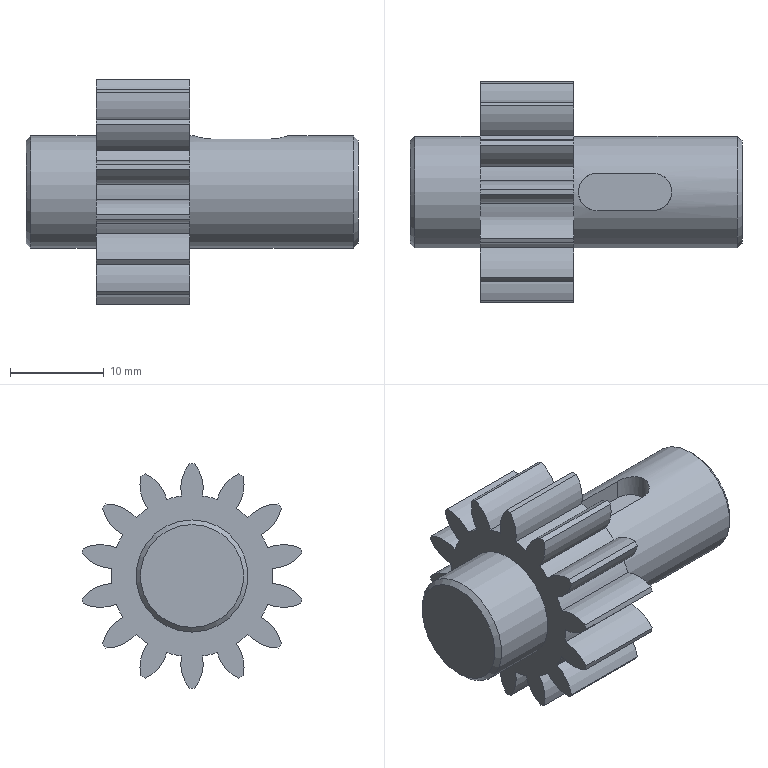Part | NX | features BREP 1 | 1 solid | 69 faces | box 35.5 x 23.519 x 24 mm | volume 6053 mm3 | cylinder 60 | plane 7 | cone 2 | commonest cylinder face diameters 8.4 x28 17.248 x14 24 x14 4 x2 12 x2